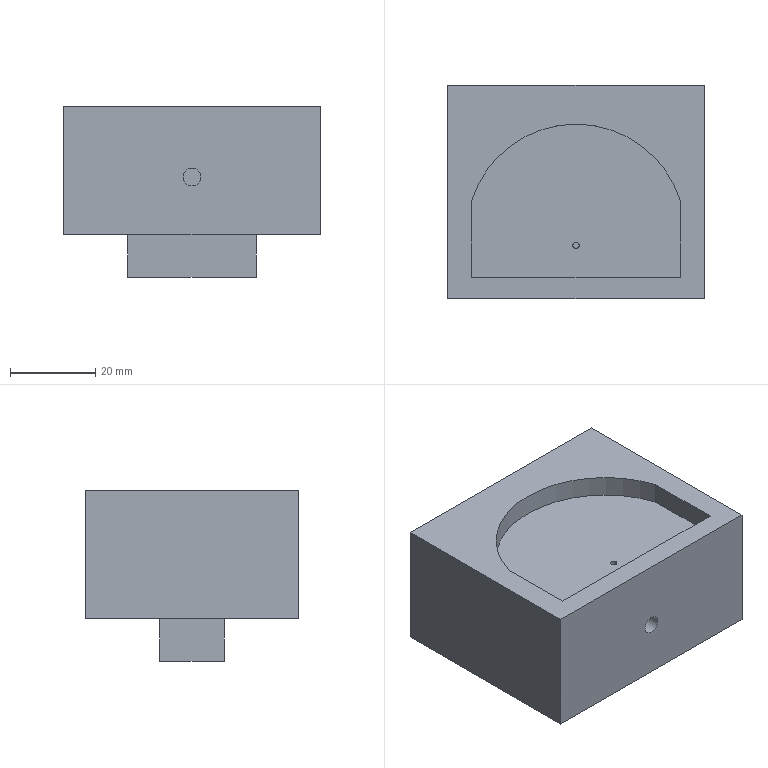Part | NX | features DATUM_CSYS 6, EXTRUDE 5, SKETCH 5 | 1 solid | 21 faces | box 60 x 50 x 40 mm | volume 86677 mm3 | plane 17 | cylinder 4 | commonest cylinder face diameters 1.5 x2 4.2 x1 51.185 x1
STEP:
#1=CARTESIAN_POINT('',(-15.,7.5,0.));
#2=VERTEX_POINT('',#1);
#3=CARTESIAN_POINT('',(-15.,-7.5,0.));
#4=VERTEX_POINT('',#3);
#5=CARTESIAN_POINT('',(-15.,7.5,0.));
#6=DIRECTION('',(0.,-1.,0.));
#7=VECTOR('',#6,1000.);
#8=LINE('',#5,#7);
#9=EDGE_CURVE('',#2,#4,#8,.T.);
#10=ORIENTED_EDGE('',*,*,#9,.T.);
#11=CARTESIAN_POINT('',(-15.,-7.5,10.));
#12=VERTEX_POINT('',#11);
#13=CARTESIAN_POINT('',(-15.,-7.5,10.));
#14=DIRECTION('',(0.,0.,-1.));
#15=VECTOR('',#14,1000.);
#16=LINE('',#13,#15);
#17=EDGE_CURVE('',#12,#4,#16,.T.);
#18=ORIENTED_EDGE('',*,*,#17,.F.);
#19=CARTESIAN_POINT('',(-15.,7.5,10.));
#20=VERTEX_POINT('',#19);
#21=CARTESIAN_POINT('',(-15.,7.5,10.));
#22=DIRECTION('',(0.,-1.,0.));
#23=VECTOR('',#22,1000.);
#24=LINE('',#21,#23);
#25=EDGE_CURVE('',#20,#12,#24,.T.);
#26=ORIENTED_EDGE('',*,*,#25,.F.);
#27=CARTESIAN_POINT('',(-15.,7.5,10.));
#28=DIRECTION('',(0.,0.,-1.));
#29=VECTOR('',#28,1000.);
#30=LINE('',#27,#29);
#31=EDGE_CURVE('',#20,#2,#30,.T.);
#32=ORIENTED_EDGE('',*,*,#31,.T.);
#33=EDGE_LOOP('',(#10,#18,#26,#32));
#34=FACE_BOUND('',#33,.T.);
#35=CARTESIAN_POINT('',(-15.,7.5,10.));
#36=DIRECTION('',(1.,0.,0.));
#37=DIRECTION('',(0.,1.,0.));
#38=AXIS2_PLACEMENT_3D('',#35,#36,#37);
#39=PLANE('',#38);
#40=ADVANCED_FACE('',(#34),#39,.F.);
#41=CARTESIAN_POINT('',(15.,-7.5,0.));
#42=VERTEX_POINT('',#41);
#43=CARTESIAN_POINT('',(-15.,-7.5,0.));
#44=DIRECTION('',(1.,0.,0.));
#45=VECTOR('',#44,1000.);
#46=LINE('',#43,#45);
#47=EDGE_CURVE('',#4,#42,#46,.T.);
#48=ORIENTED_EDGE('',*,*,#47,.T.);
#49=CARTESIAN_POINT('',(15.,-7.5,10.));
#50=VERTEX_POINT('',#49);
#51=CARTESIAN_POINT('',(15.,-7.5,10.));
#52=DIRECTION('',(0.,0.,-1.));
#53=VECTOR('',#52,1000.);
#54=LINE('',#51,#53);
#55=EDGE_CURVE('',#50,#42,#54,.T.);
#56=ORIENTED_EDGE('',*,*,#55,.F.);
#57=CARTESIAN_POINT('',(-15.,-7.5,10.));
#58=DIRECTION('',(1.,0.,0.));
#59=VECTOR('',#58,1000.);
#60=LINE('',#57,#59);
#61=EDGE_CURVE('',#12,#50,#60,.T.);
#62=ORIENTED_EDGE('',*,*,#61,.F.);
#63=ORIENTED_EDGE('',*,*,#17,.T.);
#64=EDGE_LOOP('',(#48,#56,#62,#63));
#65=FACE_BOUND('',#64,.T.);
#66=CARTESIAN_POINT('',(-15.,-7.5,10.));
#67=DIRECTION('',(0.,1.,0.));
#68=DIRECTION('',(0.,0.,1.));
#69=AXIS2_PLACEMENT_3D('',#66,#67,#68);
#70=PLANE('',#69);
#71=ADVANCED_FACE('',(#65),#70,.F.);
#72=CARTESIAN_POINT('',(15.,7.5,0.));
#73=VERTEX_POINT('',#72);
#74=CARTESIAN_POINT('',(15.,-7.5,0.));
#75=DIRECTION('',(0.,1.,0.));
#76=VECTOR('',#75,1000.);
#77=LINE('',#74,#76);
#78=EDGE_CURVE('',#42,#73,#77,.T.);
#79=ORIENTED_EDGE('',*,*,#78,.T.);
#80=CARTESIAN_POINT('',(15.,7.5,10.));
#81=VERTEX_POINT('',#80);
#82=CARTESIAN_POINT('',(15.,7.5,10.));
#83=DIRECTION('',(0.,0.,-1.));
#84=VECTOR('',#83,1000.);
#85=LINE('',#82,#84);
#86=EDGE_CURVE('',#81,#73,#85,.T.);
#87=ORIENTED_EDGE('',*,*,#86,.F.);
#88=CARTESIAN_POINT('',(15.,-7.5,10.));
#89=DIRECTION('',(0.,1.,0.));
#90=VECTOR('',#89,1000.);
#91=LINE('',#88,#90);
#92=EDGE_CURVE('',#50,#81,#91,.T.);
#93=ORIENTED_EDGE('',*,*,#92,.F.);
#94=ORIENTED_EDGE('',*,*,#55,.T.);
#95=EDGE_LOOP('',(#79,#87,#93,#94));
#96=FACE_BOUND('',#95,.T.);
#97=CARTESIAN_POINT('',(15.,-7.5,10.));
#98=DIRECTION('',(-1.,0.,0.));
#99=DIRECTION('',(0.,-1.,0.));
#100=AXIS2_PLACEMENT_3D('',#97,#98,#99);
#101=PLANE('',#100);
#102=ADVANCED_FACE('',(#96),#101,.F.);
#103=CARTESIAN_POINT('',(15.,7.5,0.));
#104=DIRECTION('',(-1.,0.,0.));
#105=VECTOR('',#104,1000.);
#106=LINE('',#103,#105);
#107=EDGE_CURVE('',#73,#2,#106,.T.);
#108=ORIENTED_EDGE('',*,*,#107,.T.);
#109=ORIENTED_EDGE('',*,*,#31,.F.);
#110=CARTESIAN_POINT('',(15.,7.5,10.));
#111=DIRECTION('',(-1.,0.,0.));
#112=VECTOR('',#111,1000.);
#113=LINE('',#110,#112);
#114=EDGE_CURVE('',#81,#20,#113,.T.);
#115=ORIENTED_EDGE('',*,*,#114,.F.);
#116=ORIENTED_EDGE('',*,*,#86,.T.);
#117=EDGE_LOOP('',(#108,#109,#115,#116));
#118=FACE_BOUND('',#117,.T.);
#119=CARTESIAN_POINT('',(15.,7.5,10.));
#120=DIRECTION('',(0.,-1.,0.));
#121=DIRECTION('',(0.,0.,-1.));
#122=AXIS2_PLACEMENT_3D('',#119,#120,#121);
#123=PLANE('',#122);
#124=ADVANCED_FACE('',(#118),#123,.F.);
#125=ORIENTED_EDGE('',*,*,#9,.F.);
#126=ORIENTED_EDGE('',*,*,#107,.F.);
#127=ORIENTED_EDGE('',*,*,#78,.F.);
#128=ORIENTED_EDGE('',*,*,#47,.F.);
#129=EDGE_LOOP('',(#125,#126,#127,#128));
#130=FACE_BOUND('',#129,.T.);
#131=CARTESIAN_POINT('',(0.,0.,0.));
#132=DIRECTION('',(0.,0.,1.));
#133=DIRECTION('',(1.,0.,0.));
#134=AXIS2_PLACEMENT_3D('',#131,#132,#133);
#135=PLANE('',#134);
#136=ADVANCED_FACE('',(#130),#135,.F.);
#137=CARTESIAN_POINT('',(-30.,25.,10.));
#138=VERTEX_POINT('',#137);
#139=CARTESIAN_POINT('',(-30.,-25.,10.));
#140=VERTEX_POINT('',#139);
#141=CARTESIAN_POINT('',(-30.,25.,10.));
#142=DIRECTION('',(0.,-1.,0.));
#143=VECTOR('',#142,1000.);
#144=LINE('',#141,#143);
#145=EDGE_CURVE('',#138,#140,#144,.T.);
#146=ORIENTED_EDGE('',*,*,#145,.F.);
#147=CARTESIAN_POINT('',(30.,25.,10.));
#148=VERTEX_POINT('',#147);
#149=CARTESIAN_POINT('',(30.,25.,10.));
#150=DIRECTION('',(-1.,0.,0.));
#151=VECTOR('',#150,1000.);
#152=LINE('',#149,#151);
#153=EDGE_CURVE('',#148,#138,#152,.T.);
#154=ORIENTED_EDGE('',*,*,#153,.F.);
#155=CARTESIAN_POINT('',(30.,-25.,10.));
#156=VERTEX_POINT('',#155);
#157=CARTESIAN_POINT('',(30.,-25.,10.));
#158=DIRECTION('',(0.,1.,0.));
#159=VECTOR('',#158,1000.);
#160=LINE('',#157,#159);
#161=EDGE_CURVE('',#156,#148,#160,.T.);
#162=ORIENTED_EDGE('',*,*,#161,.F.);
#163=CARTESIAN_POINT('',(-30.,-25.,10.));
#164=DIRECTION('',(1.,0.,0.));
#165=VECTOR('',#164,1000.);
#166=LINE('',#163,#165);
#167=EDGE_CURVE('',#140,#156,#166,.T.);
#168=ORIENTED_EDGE('',*,*,#167,.F.);
#169=EDGE_LOOP('',(#146,#154,#162,#168));
#170=FACE_BOUND('',#169,.T.);
#171=ORIENTED_EDGE('',*,*,#114,.T.);
#172=ORIENTED_EDGE('',*,*,#25,.T.);
#173=ORIENTED_EDGE('',*,*,#61,.T.);
#174=ORIENTED_EDGE('',*,*,#92,.T.);
#175=EDGE_LOOP('',(#171,#172,#173,#174));
#176=FACE_BOUND('',#175,.T.);
#177=CARTESIAN_POINT('',(0.,0.,10.));
#178=DIRECTION('',(0.,0.,1.));
#179=DIRECTION('',(1.,0.,0.));
#180=AXIS2_PLACEMENT_3D('',#177,#178,#179);
#181=PLANE('',#180);
#182=ADVANCED_FACE('',(#170,#176),#181,.F.);
#183=ORIENTED_EDGE('',*,*,#145,.T.);
#184=CARTESIAN_POINT('',(-30.,-25.,40.));
#185=VERTEX_POINT('',#184);
#186=CARTESIAN_POINT('',(-30.,-25.,40.));
#187=DIRECTION('',(0.,0.,-1.));
#188=VECTOR('',#187,1000.);
#189=LINE('',#186,#188);
#190=EDGE_CURVE('',#185,#140,#189,.T.);
#191=ORIENTED_EDGE('',*,*,#190,.F.);
#192=CARTESIAN_POINT('',(-30.,25.,40.));
#193=VERTEX_POINT('',#192);
#194=CARTESIAN_POINT('',(-30.,25.,40.));
#195=DIRECTION('',(0.,-1.,0.));
#196=VECTOR('',#195,1000.);
#197=LINE('',#194,#196);
#198=EDGE_CURVE('',#193,#185,#197,.T.);
#199=ORIENTED_EDGE('',*,*,#198,.F.);
#200=CARTESIAN_POINT('',(-30.,25.,40.));
#201=DIRECTION('',(0.,0.,-1.));
#202=VECTOR('',#201,1000.);
#203=LINE('',#200,#202);
#204=EDGE_CURVE('',#193,#138,#203,.T.);
#205=ORIENTED_EDGE('',*,*,#204,.T.);
#206=EDGE_LOOP('',(#183,#191,#199,#205));
#207=FACE_BOUND('',#206,.T.);
#208=CARTESIAN_POINT('',(-30.,25.,40.));
#209=DIRECTION('',(1.,0.,0.));
#210=DIRECTION('',(0.,1.,0.));
#211=AXIS2_PLACEMENT_3D('',#208,#209,#210);
#212=PLANE('',#211);
#213=ADVANCED_FACE('',(#207),#212,.F.);
#214=CARTESIAN_POINT('',(2.1,-25.,23.5));
#215=VERTEX_POINT('',#214);
#216=CARTESIAN_POINT('',(0.,-25.,23.5));
#217=DIRECTION('',(0.,-1.,0.));
#218=DIRECTION('',(1.,0.,0.));
#219=AXIS2_PLACEMENT_3D('',#216,#217,#218);
#220=CIRCLE('',#219,2.1);
#221=EDGE_CURVE('',#215,#215,#220,.T.);
#222=ORIENTED_EDGE('',*,*,#221,.F.);
#223=EDGE_LOOP('',(#222));
#224=FACE_BOUND('',#223,.T.);
#225=ORIENTED_EDGE('',*,*,#167,.T.);
#226=CARTESIAN_POINT('',(30.,-25.,40.));
#227=VERTEX_POINT('',#226);
#228=CARTESIAN_POINT('',(30.,-25.,40.));
#229=DIRECTION('',(0.,0.,-1.));
#230=VECTOR('',#229,1000.);
#231=LINE('',#228,#230);
#232=EDGE_CURVE('',#227,#156,#231,.T.);
#233=ORIENTED_EDGE('',*,*,#232,.F.);
#234=CARTESIAN_POINT('',(-30.,-25.,40.));
#235=DIRECTION('',(1.,0.,0.));
#236=VECTOR('',#235,1000.);
#237=LINE('',#234,#236);
#238=EDGE_CURVE('',#185,#227,#237,.T.);
#239=ORIENTED_EDGE('',*,*,#238,.F.);
#240=ORIENTED_EDGE('',*,*,#190,.T.);
#241=EDGE_LOOP('',(#225,#233,#239,#240));
#242=FACE_BOUND('',#241,.T.);
#243=CARTESIAN_POINT('',(-30.,-25.,40.));
#244=DIRECTION('',(0.,1.,0.));
#245=DIRECTION('',(-1.,0.,0.));
#246=AXIS2_PLACEMENT_3D('',#243,#244,#245);
#247=PLANE('',#246);
#248=ADVANCED_FACE('',(#224,#242),#247,.F.);
#249=ORIENTED_EDGE('',*,*,#161,.T.);
#250=CARTESIAN_POINT('',(30.,25.,40.));
#251=VERTEX_POINT('',#250);
#252=CARTESIAN_POINT('',(30.,25.,40.));
#253=DIRECTION('',(0.,0.,-1.));
#254=VECTOR('',#253,1000.);
#255=LINE('',#252,#254);
#256=EDGE_CURVE('',#251,#148,#255,.T.);
#257=ORIENTED_EDGE('',*,*,#256,.F.);
#258=CARTESIAN_POINT('',(30.,-25.,40.));
#259=DIRECTION('',(0.,1.,0.));
#260=VECTOR('',#259,1000.);
#261=LINE('',#258,#260);
#262=EDGE_CURVE('',#227,#251,#261,.T.);
#263=ORIENTED_EDGE('',*,*,#262,.F.);
#264=ORIENTED_EDGE('',*,*,#232,.T.);
#265=EDGE_LOOP('',(#249,#257,#263,#264));
#266=FACE_BOUND('',#265,.T.);
#267=CARTESIAN_POINT('',(30.,-25.,40.));
#268=DIRECTION('',(-1.,0.,0.));
#269=DIRECTION('',(0.,-1.,0.));
#270=AXIS2_PLACEMENT_3D('',#267,#268,#269);
#271=PLANE('',#270);
#272=ADVANCED_FACE('',(#266),#271,.F.);
#273=ORIENTED_EDGE('',*,*,#153,.T.);
#274=ORIENTED_EDGE('',*,*,#204,.F.);
#275=CARTESIAN_POINT('',(30.,25.,40.));
#276=DIRECTION('',(-1.,0.,0.));
#277=VECTOR('',#276,1000.);
#278=LINE('',#275,#277);
#279=EDGE_CURVE('',#251,#193,#278,.T.);
#280=ORIENTED_EDGE('',*,*,#279,.F.);
#281=ORIENTED_EDGE('',*,*,#256,.T.);
#282=EDGE_LOOP('',(#273,#274,#280,#281));
#283=FACE_BOUND('',#282,.T.);
#284=CARTESIAN_POINT('',(30.,25.,40.));
#285=DIRECTION('',(0.,-1.,0.));
#286=DIRECTION('',(1.,0.,0.));
#287=AXIS2_PLACEMENT_3D('',#284,#285,#286);
#288=PLANE('',#287);
#289=ADVANCED_FACE('',(#283),#288,.F.);
#290=CARTESIAN_POINT('',(-24.421,-2.062,40.));
#291=VERTEX_POINT('',#290);
#292=CARTESIAN_POINT('',(-24.421,-20.,40.));
#293=VERTEX_POINT('',#292);
#294=CARTESIAN_POINT('',(-24.421,-2.062,40.));
#295=DIRECTION('',(0.,-1.,0.));
#296=VECTOR('',#295,1000.);
#297=LINE('',#294,#296);
#298=EDGE_CURVE('',#291,#293,#297,.T.);
#299=ORIENTED_EDGE('',*,*,#298,.F.);
#300=CARTESIAN_POINT('',(24.421,-2.062,40.));
#301=VERTEX_POINT('',#300);
#302=CARTESIAN_POINT('',(0.,-9.716,40.));
#303=DIRECTION('',(0.,0.,1.));
#304=DIRECTION('',(1.,0.,0.));
#305=AXIS2_PLACEMENT_3D('',#302,#303,#304);
#306=CIRCLE('',#305,25.592);
#307=EDGE_CURVE('',#301,#291,#306,.T.);
#308=ORIENTED_EDGE('',*,*,#307,.F.);
#309=CARTESIAN_POINT('',(24.421,-20.,40.));
#310=VERTEX_POINT('',#309);
#311=CARTESIAN_POINT('',(24.421,-20.,40.));
#312=DIRECTION('',(0.,1.,0.));
#313=VECTOR('',#312,1000.);
#314=LINE('',#311,#313);
#315=EDGE_CURVE('',#310,#301,#314,.T.);
#316=ORIENTED_EDGE('',*,*,#315,.F.);
#317=CARTESIAN_POINT('',(-24.421,-20.,40.));
#318=DIRECTION('',(1.,0.,0.));
#319=VECTOR('',#318,1000.);
#320=LINE('',#317,#319);
#321=EDGE_CURVE('',#293,#310,#320,.T.);
#322=ORIENTED_EDGE('',*,*,#321,.F.);
#323=EDGE_LOOP('',(#299,#308,#316,#322));
#324=FACE_BOUND('',#323,.T.);
#325=ORIENTED_EDGE('',*,*,#198,.T.);
#326=ORIENTED_EDGE('',*,*,#238,.T.);
#327=ORIENTED_EDGE('',*,*,#262,.T.);
#328=ORIENTED_EDGE('',*,*,#279,.T.);
#329=EDGE_LOOP('',(#325,#326,#327,#328));
#330=FACE_BOUND('',#329,.T.);
#331=CARTESIAN_POINT('',(0.,0.,40.));
#332=DIRECTION('',(0.,0.,1.));
#333=DIRECTION('',(1.,0.,0.));
#334=AXIS2_PLACEMENT_3D('',#331,#332,#333);
#335=PLANE('',#334);
#336=ADVANCED_FACE('',(#324,#330),#335,.T.);
#337=ORIENTED_EDGE('',*,*,#298,.T.);
#338=CARTESIAN_POINT('',(-24.421,-20.,35.));
#339=VERTEX_POINT('',#338);
#340=CARTESIAN_POINT('',(-24.421,-20.,35.));
#341=DIRECTION('',(0.,0.,1.));
#342=VECTOR('',#341,1000.);
#343=LINE('',#340,#342);
#344=EDGE_CURVE('',#293,#339,#343,.F.);
#345=ORIENTED_EDGE('',*,*,#344,.T.);
#346=CARTESIAN_POINT('',(-24.421,-2.062,35.));
#347=VERTEX_POINT('',#346);
#348=CARTESIAN_POINT('',(-24.421,-2.062,35.));
#349=DIRECTION('',(0.,-1.,0.));
#350=VECTOR('',#349,1000.);
#351=LINE('',#348,#350);
#352=EDGE_CURVE('',#339,#347,#351,.F.);
#353=ORIENTED_EDGE('',*,*,#352,.T.);
#354=CARTESIAN_POINT('',(-24.421,-2.062,35.));
#355=DIRECTION('',(0.,0.,1.));
#356=VECTOR('',#355,1000.);
#357=LINE('',#354,#356);
#358=EDGE_CURVE('',#291,#347,#357,.F.);
#359=ORIENTED_EDGE('',*,*,#358,.F.);
#360=EDGE_LOOP('',(#337,#345,#353,#359));
#361=FACE_BOUND('',#360,.T.);
#362=CARTESIAN_POINT('',(-24.421,-2.062,35.));
#363=DIRECTION('',(-1.,0.,0.));
#364=DIRECTION('',(0.,-1.,0.));
#365=AXIS2_PLACEMENT_3D('',#362,#363,#364);
#366=PLANE('',#365);
#367=ADVANCED_FACE('',(#361),#366,.F.);
#368=ORIENTED_EDGE('',*,*,#321,.T.);
#369=CARTESIAN_POINT('',(24.421,-20.,35.));
#370=VERTEX_POINT('',#369);
#371=CARTESIAN_POINT('',(24.421,-20.,35.));
#372=DIRECTION('',(0.,0.,1.));
#373=VECTOR('',#372,1000.);
#374=LINE('',#371,#373);
#375=EDGE_CURVE('',#310,#370,#374,.F.);
#376=ORIENTED_EDGE('',*,*,#375,.T.);
#377=CARTESIAN_POINT('',(-24.421,-20.,35.));
#378=DIRECTION('',(1.,0.,0.));
#379=VECTOR('',#378,1000.);
#380=LINE('',#377,#379);
#381=EDGE_CURVE('',#370,#339,#380,.F.);
#382=ORIENTED_EDGE('',*,*,#381,.T.);
#383=ORIENTED_EDGE('',*,*,#344,.F.);
#384=EDGE_LOOP('',(#368,#376,#382,#383));
#385=FACE_BOUND('',#384,.T.);
#386=CARTESIAN_POINT('',(-24.421,-20.,35.));
#387=DIRECTION('',(0.,-1.,0.));
#388=DIRECTION('',(1.,0.,0.));
#389=AXIS2_PLACEMENT_3D('',#386,#387,#388);
#390=PLANE('',#389);
#391=ADVANCED_FACE('',(#385),#390,.F.);
#392=ORIENTED_EDGE('',*,*,#315,.T.);
#393=CARTESIAN_POINT('',(24.421,-2.062,35.));
#394=VERTEX_POINT('',#393);
#395=CARTESIAN_POINT('',(24.421,-2.062,35.));
#396=DIRECTION('',(0.,0.,1.));
#397=VECTOR('',#396,1000.);
#398=LINE('',#395,#397);
#399=EDGE_CURVE('',#301,#394,#398,.F.);
#400=ORIENTED_EDGE('',*,*,#399,.T.);
#401=CARTESIAN_POINT('',(24.421,-20.,35.));
#402=DIRECTION('',(0.,1.,0.));
#403=VECTOR('',#402,1000.);
#404=LINE('',#401,#403);
#405=EDGE_CURVE('',#394,#370,#404,.F.);
#406=ORIENTED_EDGE('',*,*,#405,.T.);
#407=ORIENTED_EDGE('',*,*,#375,.F.);
#408=EDGE_LOOP('',(#392,#400,#406,#407));
#409=FACE_BOUND('',#408,.T.);
#410=CARTESIAN_POINT('',(24.421,-20.,35.));
#411=DIRECTION('',(1.,0.,0.));
#412=DIRECTION('',(0.,1.,0.));
#413=AXIS2_PLACEMENT_3D('',#410,#411,#412);
#414=PLANE('',#413);
#415=ADVANCED_FACE('',(#409),#414,.F.);
#416=ORIENTED_EDGE('',*,*,#307,.T.);
#417=ORIENTED_EDGE('',*,*,#358,.T.);
#418=CARTESIAN_POINT('',(0.,-9.716,35.));
#419=DIRECTION('',(0.,0.,1.));
#420=DIRECTION('',(-1.,0.,0.));
#421=AXIS2_PLACEMENT_3D('',#418,#419,#420);
#422=CIRCLE('',#421,25.592);
#423=EDGE_CURVE('',#347,#394,#422,.F.);
#424=ORIENTED_EDGE('',*,*,#423,.T.);
#425=ORIENTED_EDGE('',*,*,#399,.F.);
#426=EDGE_LOOP('',(#416,#417,#424,#425));
#427=FACE_BOUND('',#426,.T.);
#428=CARTESIAN_POINT('',(0.,-9.716,35.));
#429=DIRECTION('',(0.,0.,1.));
#430=DIRECTION('',(1.,0.,0.));
#431=AXIS2_PLACEMENT_3D('',#428,#429,#430);
#432=CYLINDRICAL_SURFACE('',#431,25.592);
#433=ADVANCED_FACE('',(#427),#432,.F.);
#434=CARTESIAN_POINT('',(-0.75,-12.5,35.));
#435=VERTEX_POINT('',#434);
#436=CARTESIAN_POINT('',(0.,-12.5,35.));
#437=DIRECTION('',(0.,0.,1.));
#438=DIRECTION('',(-1.,0.,0.));
#439=AXIS2_PLACEMENT_3D('',#436,#437,#438);
#440=CIRCLE('',#439,0.75);
#441=EDGE_CURVE('',#435,#435,#440,.T.);
#442=ORIENTED_EDGE('',*,*,#441,.F.);
#443=EDGE_LOOP('',(#442));
#444=FACE_BOUND('',#443,.T.);
#445=ORIENTED_EDGE('',*,*,#352,.F.);
#446=ORIENTED_EDGE('',*,*,#381,.F.);
#447=ORIENTED_EDGE('',*,*,#405,.F.);
#448=ORIENTED_EDGE('',*,*,#423,.F.);
#449=EDGE_LOOP('',(#445,#446,#447,#448));
#450=FACE_BOUND('',#449,.T.);
#451=CARTESIAN_POINT('',(0.,-9.716,35.));
#452=DIRECTION('',(0.,0.,1.));
#453=DIRECTION('',(1.,0.,0.));
#454=AXIS2_PLACEMENT_3D('',#451,#452,#453);
#455=PLANE('',#454);
#456=ADVANCED_FACE('',(#444,#450),#455,.T.);
#457=CARTESIAN_POINT('',(0.75,-12.5,25.462));
#458=VERTEX_POINT('',#457);
#459=CARTESIAN_POINT('',(0.0002963,-11.375,25.738));
#460=CARTESIAN_POINT('',(1.125,-12.5,25.323));
#461=CARTESIAN_POINT('',(0.0009005,-13.625,25.738));
#462=CARTESIAN_POINT('',(-1.125,-12.501,25.323));
#463=CARTESIAN_POINT('',(0.0002963,-11.375,25.738));
#464=CARTESIAN_POINT('',(1.125,-12.5,25.323));
#465=CARTESIAN_POINT('',(0.0009005,-13.625,25.738));
#466=B_SPLINE_CURVE_WITH_KNOTS('',3,(#459,#460,#461,#462,#463,#464,#465),.UNSPECIFIED.,.T.,.F.,(1,1,1,1,1,1,1,1,1,1,1),(-0.003546,-0.002364,-0.001182,0.,0.001182,0.002364,0.003546,0.004728,0.00591,0.007093,0.008275),.UNSPECIFIED.);
#467=EDGE_CURVE('',#458,#458,#466,.T.);
#468=ORIENTED_EDGE('',*,*,#467,.T.);
#469=EDGE_LOOP('',(#468));
#470=FACE_BOUND('',#469,.T.);
#471=ORIENTED_EDGE('',*,*,#441,.T.);
#472=EDGE_LOOP('',(#471));
#473=FACE_BOUND('',#472,.T.);
#474=CARTESIAN_POINT('',(0.,-12.5,20.));
#475=DIRECTION('',(0.,0.,1.));
#476=DIRECTION('',(1.,0.,0.));
#477=AXIS2_PLACEMENT_3D('',#474,#475,#476);
#478=CYLINDRICAL_SURFACE('',#477,0.75);
#479=ADVANCED_FACE('',(#470,#473),#478,.F.);
#480=ORIENTED_EDGE('',*,*,#467,.F.);
#481=EDGE_LOOP('',(#480));
#482=FACE_BOUND('',#481,.T.);
#483=CARTESIAN_POINT('',(2.1,-10.,23.5));
#484=VERTEX_POINT('',#483);
#485=CARTESIAN_POINT('',(0.,-10.,23.5));
#486=DIRECTION('',(0.,-1.,0.));
#487=DIRECTION('',(1.,0.,0.));
#488=AXIS2_PLACEMENT_3D('',#485,#486,#487);
#489=CIRCLE('',#488,2.1);
#490=EDGE_CURVE('',#484,#484,#489,.F.);
#491=ORIENTED_EDGE('',*,*,#490,.T.);
#492=EDGE_LOOP('',(#491));
#493=FACE_BOUND('',#492,.T.);
#494=ORIENTED_EDGE('',*,*,#221,.T.);
#495=EDGE_LOOP('',(#494));
#496=FACE_BOUND('',#495,.T.);
#497=CARTESIAN_POINT('',(0.75,-12.5,21.538));
#498=VERTEX_POINT('',#497);
#499=CARTESIAN_POINT('',(0.0002963,-13.625,21.262));
#500=CARTESIAN_POINT('',(1.125,-12.5,21.677));
#501=CARTESIAN_POINT('',(0.0009005,-11.375,21.262));
#502=CARTESIAN_POINT('',(-1.125,-12.499,21.677));
#503=CARTESIAN_POINT('',(0.0002963,-13.625,21.262));
#504=CARTESIAN_POINT('',(1.125,-12.5,21.677));
#505=CARTESIAN_POINT('',(0.0009005,-11.375,21.262));
#506=B_SPLINE_CURVE_WITH_KNOTS('',3,(#499,#500,#501,#502,#503,#504,#505),.UNSPECIFIED.,.T.,.F.,(1,1,1,1,1,1,1,1,1,1,1),(-0.003546,-0.002364,-0.001182,0.,0.001182,0.002364,0.003546,0.004728,0.00591,0.007093,0.008275),.UNSPECIFIED.);
#507=EDGE_CURVE('',#498,#498,#506,.T.);
#508=ORIENTED_EDGE('',*,*,#507,.F.);
#509=EDGE_LOOP('',(#508));
#510=FACE_BOUND('',#509,.T.);
#511=CARTESIAN_POINT('',(0.,-10.,23.5));
#512=DIRECTION('',(0.,-1.,0.));
#513=DIRECTION('',(0.,0.,-1.));
#514=AXIS2_PLACEMENT_3D('',#511,#512,#513);
#515=CYLINDRICAL_SURFACE('',#514,2.1);
#516=ADVANCED_FACE('',(#482,#493,#496,#510),#515,.F.);
#517=ORIENTED_EDGE('',*,*,#490,.F.);
#518=EDGE_LOOP('',(#517));
#519=FACE_BOUND('',#518,.T.);
#520=CARTESIAN_POINT('',(0.,-10.,23.5));
#521=DIRECTION('',(0.,-1.,0.));
#522=DIRECTION('',(0.,0.,-1.));
#523=AXIS2_PLACEMENT_3D('',#520,#521,#522);
#524=PLANE('',#523);
#525=ADVANCED_FACE('',(#519),#524,.T.);
#526=CARTESIAN_POINT('',(-0.75,-12.5,20.));
#527=VERTEX_POINT('',#526);
#528=CARTESIAN_POINT('',(0.,-12.5,20.));
#529=DIRECTION('',(0.,0.,1.));
#530=DIRECTION('',(-1.,0.,0.));
#531=AXIS2_PLACEMENT_3D('',#528,#529,#530);
#532=CIRCLE('',#531,0.75);
#533=EDGE_CURVE('',#527,#527,#532,.F.);
#534=ORIENTED_EDGE('',*,*,#533,.F.);
#535=EDGE_LOOP('',(#534));
#536=FACE_BOUND('',#535,.T.);
#537=CARTESIAN_POINT('',(0.,-12.5,20.));
#538=DIRECTION('',(0.,0.,1.));
#539=DIRECTION('',(1.,0.,0.));
#540=AXIS2_PLACEMENT_3D('',#537,#538,#539);
#541=PLANE('',#540);
#542=ADVANCED_FACE('',(#536),#541,.T.);
#543=ORIENTED_EDGE('',*,*,#507,.T.);
#544=EDGE_LOOP('',(#543));
#545=FACE_BOUND('',#544,.T.);
#546=ORIENTED_EDGE('',*,*,#533,.T.);
#547=EDGE_LOOP('',(#546));
#548=FACE_BOUND('',#547,.T.);
#549=CARTESIAN_POINT('',(0.,-12.5,20.));
#550=DIRECTION('',(0.,0.,1.));
#551=DIRECTION('',(1.,0.,0.));
#552=AXIS2_PLACEMENT_3D('',#549,#550,#551);
#553=CYLINDRICAL_SURFACE('',#552,0.75);
#554=ADVANCED_FACE('',(#545,#548),#553,.F.);
#555=CLOSED_SHELL('',(#40,#71,#102,#124,#136,#182,#213,#248,#272,#289,#336,#367,#391,#415,#433,#456,#479,#516,#525,#542,#554));
#556=MANIFOLD_SOLID_BREP('',#555);
#557=(LENGTH_UNIT()NAMED_UNIT(*)SI_UNIT(.MILLI.,.METRE.));
#558=UNCERTAINTY_MEASURE_WITH_UNIT(LENGTH_MEASURE(0.0508),#557,'','');
#559=(NAMED_UNIT(*)PLANE_ANGLE_UNIT()SI_UNIT($,.RADIAN.));
#560=(NAMED_UNIT(*)SI_UNIT($,.STERADIAN.)SOLID_ANGLE_UNIT());
#561=(GEOMETRIC_REPRESENTATION_CONTEXT(3)GLOBAL_UNCERTAINTY_ASSIGNED_CONTEXT((#558))GLOBAL_UNIT_ASSIGNED_CONTEXT((#557,#559,#560))REPRESENTATION_CONTEXT('',''));
#562=ADVANCED_BREP_SHAPE_REPRESENTATION('',(#556),#561);